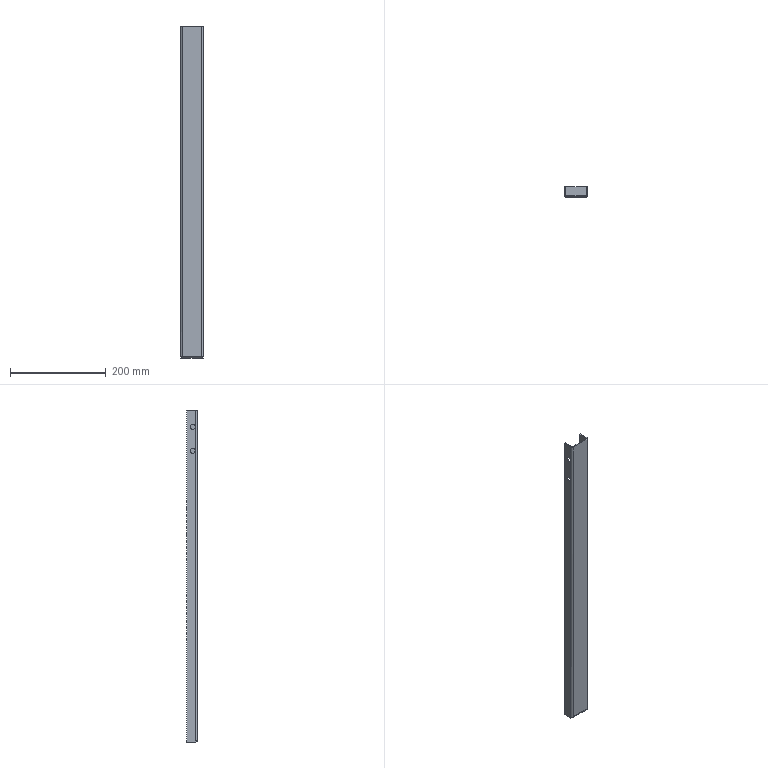Part | NX | features solid 2 | 1 solid | 34 faces | box 48 x 23 x 695 mm | volume 122908 mm3 | plane 24 | cylinder 10 | commonest cylinder face diameters 10 x4 4 x3 8 x3
STEP:
#1=CARTESIAN_POINT('',(1114.,-660.,1129.5));
#2=VERTEX_POINT('',#1);
#3=CARTESIAN_POINT('',(1114.,-670.,1129.5));
#4=VERTEX_POINT('',#3);
#5=CARTESIAN_POINT('',(1114.,-665.,1129.5));
#6=DIRECTION('',(1.,0.,0.));
#7=DIRECTION('',(0.,-1.,0.));
#8=AXIS2_PLACEMENT_3D('',#5,#6,#7);
#9=CIRCLE('',#8,5.);
#10=EDGE_CURVE('',#2,#4,#9,.T.);
#11=ORIENTED_EDGE('',*,*,#10,.F.);
#12=CARTESIAN_POINT('',(1114.,-665.,1129.5));
#13=DIRECTION('',(1.,0.,0.));
#14=DIRECTION('',(0.,-1.,0.));
#15=AXIS2_PLACEMENT_3D('',#12,#13,#14);
#16=CIRCLE('',#15,5.);
#17=EDGE_CURVE('',#4,#2,#16,.T.);
#18=ORIENTED_EDGE('',*,*,#17,.F.);
#19=EDGE_LOOP('',(#11,#18));
#20=FACE_BOUND('',#19,.T.);
#21=CARTESIAN_POINT('',(1114.,-660.,1079.5));
#22=VERTEX_POINT('',#21);
#23=CARTESIAN_POINT('',(1114.,-670.,1079.5));
#24=VERTEX_POINT('',#23);
#25=CARTESIAN_POINT('',(1114.,-665.,1079.5));
#26=DIRECTION('',(1.,0.,0.));
#27=DIRECTION('',(0.,-1.,0.));
#28=AXIS2_PLACEMENT_3D('',#25,#26,#27);
#29=CIRCLE('',#28,5.);
#30=EDGE_CURVE('',#22,#24,#29,.T.);
#31=ORIENTED_EDGE('',*,*,#30,.F.);
#32=CARTESIAN_POINT('',(1114.,-665.,1079.5));
#33=DIRECTION('',(1.,0.,0.));
#34=DIRECTION('',(0.,-1.,0.));
#35=AXIS2_PLACEMENT_3D('',#32,#33,#34);
#36=CIRCLE('',#35,5.);
#37=EDGE_CURVE('',#24,#22,#36,.T.);
#38=ORIENTED_EDGE('',*,*,#37,.F.);
#39=EDGE_LOOP('',(#31,#38));
#40=FACE_BOUND('',#39,.T.);
#41=CARTESIAN_POINT('',(1114.,-652.,470.));
#42=VERTEX_POINT('',#41);
#43=CARTESIAN_POINT('',(1114.,-671.,470.));
#44=VERTEX_POINT('',#43);
#45=CARTESIAN_POINT('',(1114.,-652.,470.));
#46=DIRECTION('',(0.,-1.,0.));
#47=VECTOR('',#46,1000.);
#48=LINE('',#45,#47);
#49=EDGE_CURVE('',#42,#44,#48,.T.);
#50=ORIENTED_EDGE('',*,*,#49,.F.);
#51=CARTESIAN_POINT('',(1114.,-652.,1165.));
#52=VERTEX_POINT('',#51);
#53=CARTESIAN_POINT('',(1114.,-652.,-140.));
#54=DIRECTION('',(0.,0.,1.));
#55=VECTOR('',#54,1000.);
#56=LINE('',#53,#55);
#57=EDGE_CURVE('',#42,#52,#56,.T.);
#58=ORIENTED_EDGE('',*,*,#57,.T.);
#59=CARTESIAN_POINT('',(1114.,-671.,1165.));
#60=VERTEX_POINT('',#59);
#61=CARTESIAN_POINT('',(1114.,-652.,1165.));
#62=DIRECTION('',(0.,1.,0.));
#63=VECTOR('',#62,1000.);
#64=LINE('',#61,#63);
#65=EDGE_CURVE('',#60,#52,#64,.T.);
#66=ORIENTED_EDGE('',*,*,#65,.F.);
#67=CARTESIAN_POINT('',(1114.,-671.,472.1));
#68=VERTEX_POINT('',#67);
#69=CARTESIAN_POINT('',(1114.,-671.,-140.));
#70=DIRECTION('',(0.,0.,1.));
#71=VECTOR('',#70,1000.);
#72=LINE('',#69,#71);
#73=EDGE_CURVE('',#68,#60,#72,.T.);
#74=ORIENTED_EDGE('',*,*,#73,.F.);
#75=CARTESIAN_POINT('',(1114.,-671.,-140.));
#76=DIRECTION('',(0.,0.,1.));
#77=VECTOR('',#76,1000.);
#78=LINE('',#75,#77);
#79=EDGE_CURVE('',#44,#68,#78,.T.);
#80=ORIENTED_EDGE('',*,*,#79,.F.);
#81=EDGE_LOOP('',(#50,#58,#66,#74,#80));
#82=FACE_BOUND('',#81,.T.);
#83=CARTESIAN_POINT('',(1114.,-652.,-140.));
#84=DIRECTION('',(1.,0.,0.));
#85=DIRECTION('',(0.,0.,1.));
#86=AXIS2_PLACEMENT_3D('',#83,#84,#85);
#87=PLANE('',#86);
#88=ADVANCED_FACE('',(#20,#40,#82),#87,.T.);
#89=CARTESIAN_POINT('',(1112.,-660.,1129.5));
#90=VERTEX_POINT('',#89);
#91=CARTESIAN_POINT('',(1112.,-670.,1129.5));
#92=VERTEX_POINT('',#91);
#93=CARTESIAN_POINT('',(1112.,-665.,1129.5));
#94=DIRECTION('',(1.,0.,0.));
#95=DIRECTION('',(0.,-1.,0.));
#96=AXIS2_PLACEMENT_3D('',#93,#94,#95);
#97=CIRCLE('',#96,5.);
#98=EDGE_CURVE('',#90,#92,#97,.T.);
#99=ORIENTED_EDGE('',*,*,#98,.T.);
#100=CARTESIAN_POINT('',(1112.,-665.,1129.5));
#101=DIRECTION('',(1.,0.,0.));
#102=DIRECTION('',(0.,-1.,0.));
#103=AXIS2_PLACEMENT_3D('',#100,#101,#102);
#104=CIRCLE('',#103,5.);
#105=EDGE_CURVE('',#92,#90,#104,.T.);
#106=ORIENTED_EDGE('',*,*,#105,.T.);
#107=EDGE_LOOP('',(#99,#106));
#108=FACE_BOUND('',#107,.T.);
#109=CARTESIAN_POINT('',(1112.,-660.,1079.5));
#110=VERTEX_POINT('',#109);
#111=CARTESIAN_POINT('',(1112.,-670.,1079.5));
#112=VERTEX_POINT('',#111);
#113=CARTESIAN_POINT('',(1112.,-665.,1079.5));
#114=DIRECTION('',(1.,0.,0.));
#115=DIRECTION('',(0.,-1.,0.));
#116=AXIS2_PLACEMENT_3D('',#113,#114,#115);
#117=CIRCLE('',#116,5.);
#118=EDGE_CURVE('',#110,#112,#117,.T.);
#119=ORIENTED_EDGE('',*,*,#118,.T.);
#120=CARTESIAN_POINT('',(1112.,-665.,1079.5));
#121=DIRECTION('',(1.,0.,0.));
#122=DIRECTION('',(0.,-1.,0.));
#123=AXIS2_PLACEMENT_3D('',#120,#121,#122);
#124=CIRCLE('',#123,5.);
#125=EDGE_CURVE('',#112,#110,#124,.T.);
#126=ORIENTED_EDGE('',*,*,#125,.T.);
#127=EDGE_LOOP('',(#119,#126));
#128=FACE_BOUND('',#127,.T.);
#129=CARTESIAN_POINT('',(1112.,-652.,470.));
#130=VERTEX_POINT('',#129);
#131=CARTESIAN_POINT('',(1112.,-652.,1165.));
#132=VERTEX_POINT('',#131);
#133=CARTESIAN_POINT('',(1112.,-652.,-140.));
#134=DIRECTION('',(0.,0.,1.));
#135=VECTOR('',#134,1000.);
#136=LINE('',#133,#135);
#137=EDGE_CURVE('',#130,#132,#136,.T.);
#138=ORIENTED_EDGE('',*,*,#137,.F.);
#139=CARTESIAN_POINT('',(1112.,-671.,470.));
#140=VERTEX_POINT('',#139);
#141=CARTESIAN_POINT('',(1112.,-652.,470.));
#142=DIRECTION('',(0.,-1.,0.));
#143=VECTOR('',#142,1000.);
#144=LINE('',#141,#143);
#145=EDGE_CURVE('',#130,#140,#144,.T.);
#146=ORIENTED_EDGE('',*,*,#145,.T.);
#147=CARTESIAN_POINT('',(1112.,-671.,472.1));
#148=VERTEX_POINT('',#147);
#149=CARTESIAN_POINT('',(1112.,-671.,-140.));
#150=DIRECTION('',(0.,0.,1.));
#151=VECTOR('',#150,1000.);
#152=LINE('',#149,#151);
#153=EDGE_CURVE('',#140,#148,#152,.T.);
#154=ORIENTED_EDGE('',*,*,#153,.T.);
#155=CARTESIAN_POINT('',(1112.,-671.,1165.));
#156=VERTEX_POINT('',#155);
#157=CARTESIAN_POINT('',(1112.,-671.,-140.));
#158=DIRECTION('',(0.,0.,1.));
#159=VECTOR('',#158,1000.);
#160=LINE('',#157,#159);
#161=EDGE_CURVE('',#148,#156,#160,.T.);
#162=ORIENTED_EDGE('',*,*,#161,.T.);
#163=CARTESIAN_POINT('',(1112.,-652.,1165.));
#164=DIRECTION('',(0.,1.,0.));
#165=VECTOR('',#164,1000.);
#166=LINE('',#163,#165);
#167=EDGE_CURVE('',#156,#132,#166,.T.);
#168=ORIENTED_EDGE('',*,*,#167,.T.);
#169=EDGE_LOOP('',(#138,#146,#154,#162,#168));
#170=FACE_BOUND('',#169,.T.);
#171=CARTESIAN_POINT('',(1112.,-652.,-140.));
#172=DIRECTION('',(1.,0.,0.));
#173=DIRECTION('',(0.,0.,1.));
#174=AXIS2_PLACEMENT_3D('',#171,#172,#173);
#175=PLANE('',#174);
#176=ADVANCED_FACE('',(#108,#128,#170),#175,.F.);
#177=ORIENTED_EDGE('',*,*,#49,.T.);
#178=CARTESIAN_POINT('',(1112.,-671.,470.));
#179=DIRECTION('',(1.,0.,0.));
#180=VECTOR('',#179,1000.);
#181=LINE('',#178,#180);
#182=EDGE_CURVE('',#140,#44,#181,.T.);
#183=ORIENTED_EDGE('',*,*,#182,.F.);
#184=ORIENTED_EDGE('',*,*,#145,.F.);
#185=CARTESIAN_POINT('',(1114.,-652.,470.));
#186=DIRECTION('',(1.,0.,0.));
#187=VECTOR('',#186,1000.);
#188=LINE('',#185,#187);
#189=EDGE_CURVE('',#130,#42,#188,.T.);
#190=ORIENTED_EDGE('',*,*,#189,.T.);
#191=EDGE_LOOP('',(#177,#183,#184,#190));
#192=FACE_BOUND('',#191,.T.);
#193=CARTESIAN_POINT('',(1158.,-673.,470.));
#194=DIRECTION('',(0.,0.,1.));
#195=DIRECTION('',(1.,0.,0.));
#196=AXIS2_PLACEMENT_3D('',#193,#194,#195);
#197=PLANE('',#196);
#198=ADVANCED_FACE('',(#192),#197,.F.);
#199=CARTESIAN_POINT('',(1110.,-670.,1079.5));
#200=DIRECTION('',(1.,0.,0.));
#201=VECTOR('',#200,1000.);
#202=LINE('',#199,#201);
#203=EDGE_CURVE('',#112,#24,#202,.T.);
#204=ORIENTED_EDGE('',*,*,#203,.F.);
#205=ORIENTED_EDGE('',*,*,#118,.F.);
#206=CARTESIAN_POINT('',(1110.,-660.,1079.5));
#207=DIRECTION('',(1.,0.,0.));
#208=VECTOR('',#207,1000.);
#209=LINE('',#206,#208);
#210=EDGE_CURVE('',#22,#110,#209,.F.);
#211=ORIENTED_EDGE('',*,*,#210,.F.);
#212=ORIENTED_EDGE('',*,*,#30,.T.);
#213=EDGE_LOOP('',(#204,#205,#211,#212));
#214=FACE_BOUND('',#213,.T.);
#215=CARTESIAN_POINT('',(1110.,-665.,1079.5));
#216=DIRECTION('',(1.,0.,0.));
#217=DIRECTION('',(0.,1.,0.));
#218=AXIS2_PLACEMENT_3D('',#215,#216,#217);
#219=CYLINDRICAL_SURFACE('',#218,5.);
#220=ADVANCED_FACE('',(#214),#219,.F.);
#221=CARTESIAN_POINT('',(1110.,-670.,1129.5));
#222=DIRECTION('',(1.,0.,0.));
#223=VECTOR('',#222,1000.);
#224=LINE('',#221,#223);
#225=EDGE_CURVE('',#4,#92,#224,.F.);
#226=ORIENTED_EDGE('',*,*,#225,.T.);
#227=ORIENTED_EDGE('',*,*,#98,.F.);
#228=CARTESIAN_POINT('',(1110.,-660.,1129.5));
#229=DIRECTION('',(1.,0.,0.));
#230=VECTOR('',#229,1000.);
#231=LINE('',#228,#230);
#232=EDGE_CURVE('',#90,#2,#231,.T.);
#233=ORIENTED_EDGE('',*,*,#232,.T.);
#234=ORIENTED_EDGE('',*,*,#10,.T.);
#235=EDGE_LOOP('',(#226,#227,#233,#234));
#236=FACE_BOUND('',#235,.T.);
#237=CARTESIAN_POINT('',(1110.,-665.,1129.5));
#238=DIRECTION('',(1.,0.,0.));
#239=DIRECTION('',(0.,1.,0.));
#240=AXIS2_PLACEMENT_3D('',#237,#238,#239);
#241=CYLINDRICAL_SURFACE('',#240,5.);
#242=ADVANCED_FACE('',(#236),#241,.F.);
#243=ORIENTED_EDGE('',*,*,#189,.F.);
#244=ORIENTED_EDGE('',*,*,#137,.T.);
#245=CARTESIAN_POINT('',(1114.,-652.,1165.));
#246=DIRECTION('',(1.,0.,0.));
#247=VECTOR('',#246,1000.);
#248=LINE('',#245,#247);
#249=EDGE_CURVE('',#132,#52,#248,.T.);
#250=ORIENTED_EDGE('',*,*,#249,.T.);
#251=ORIENTED_EDGE('',*,*,#57,.F.);
#252=EDGE_LOOP('',(#243,#244,#250,#251));
#253=FACE_BOUND('',#252,.T.);
#254=CARTESIAN_POINT('',(1114.,-652.,-140.));
#255=DIRECTION('',(0.,1.,0.));
#256=DIRECTION('',(0.,0.,-1.));
#257=AXIS2_PLACEMENT_3D('',#254,#255,#256);
#258=PLANE('',#257);
#259=ADVANCED_FACE('',(#253),#258,.T.);
#260=ORIENTED_EDGE('',*,*,#79,.T.);
#261=CARTESIAN_POINT('',(1136.,-671.,472.1));
#262=DIRECTION('',(-1.,0.,0.));
#263=VECTOR('',#262,1000.);
#264=LINE('',#261,#263);
#265=EDGE_CURVE('',#68,#148,#264,.T.);
#266=ORIENTED_EDGE('',*,*,#265,.T.);
#267=ORIENTED_EDGE('',*,*,#153,.F.);
#268=ORIENTED_EDGE('',*,*,#182,.T.);
#269=EDGE_LOOP('',(#260,#266,#267,#268));
#270=FACE_BOUND('',#269,.T.);
#271=CARTESIAN_POINT('',(1112.,-671.,-140.));
#272=DIRECTION('',(0.,1.,0.));
#273=DIRECTION('',(0.,0.,-1.));
#274=AXIS2_PLACEMENT_3D('',#271,#272,#273);
#275=PLANE('',#274);
#276=ADVANCED_FACE('',(#270),#275,.F.);
#277=CARTESIAN_POINT('',(1116.,-675.,1165.));
#278=VERTEX_POINT('',#277);
#279=CARTESIAN_POINT('',(1116.,-671.,1165.));
#280=DIRECTION('',(0.,0.,-1.));
#281=DIRECTION('',(0.,-1.,0.));
#282=AXIS2_PLACEMENT_3D('',#279,#280,#281);
#283=CIRCLE('',#282,4.);
#284=EDGE_CURVE('',#278,#156,#283,.T.);
#285=ORIENTED_EDGE('',*,*,#284,.F.);
#286=CARTESIAN_POINT('',(1156.,-675.,1165.));
#287=VERTEX_POINT('',#286);
#288=CARTESIAN_POINT('',(1114.,-675.,1165.));
#289=DIRECTION('',(-1.,0.,0.));
#290=VECTOR('',#289,1000.);
#291=LINE('',#288,#290);
#292=EDGE_CURVE('',#287,#278,#291,.T.);
#293=ORIENTED_EDGE('',*,*,#292,.F.);
#294=CARTESIAN_POINT('',(1160.,-671.,1165.));
#295=VERTEX_POINT('',#294);
#296=CARTESIAN_POINT('',(1156.,-671.,1165.));
#297=DIRECTION('',(0.,0.,-1.));
#298=DIRECTION('',(0.,-1.,0.));
#299=AXIS2_PLACEMENT_3D('',#296,#297,#298);
#300=CIRCLE('',#299,4.);
#301=EDGE_CURVE('',#295,#287,#300,.T.);
#302=ORIENTED_EDGE('',*,*,#301,.F.);
#303=CARTESIAN_POINT('',(1160.,-652.,1165.));
#304=VERTEX_POINT('',#303);
#305=CARTESIAN_POINT('',(1160.,-673.,1165.));
#306=DIRECTION('',(0.,-1.,0.));
#307=VECTOR('',#306,1000.);
#308=LINE('',#305,#307);
#309=EDGE_CURVE('',#304,#295,#308,.T.);
#310=ORIENTED_EDGE('',*,*,#309,.F.);
#311=CARTESIAN_POINT('',(1158.,-652.,1165.));
#312=VERTEX_POINT('',#311);
#313=CARTESIAN_POINT('',(1158.,-652.,1165.));
#314=DIRECTION('',(-1.,0.,0.));
#315=VECTOR('',#314,1000.);
#316=LINE('',#313,#315);
#317=EDGE_CURVE('',#304,#312,#316,.T.);
#318=ORIENTED_EDGE('',*,*,#317,.T.);
#319=CARTESIAN_POINT('',(1158.,-671.,1165.));
#320=VERTEX_POINT('',#319);
#321=CARTESIAN_POINT('',(1158.,-673.,1165.));
#322=DIRECTION('',(0.,-1.,0.));
#323=VECTOR('',#322,1000.);
#324=LINE('',#321,#323);
#325=EDGE_CURVE('',#312,#320,#324,.T.);
#326=ORIENTED_EDGE('',*,*,#325,.T.);
#327=CARTESIAN_POINT('',(1156.,-673.,1165.));
#328=VERTEX_POINT('',#327);
#329=CARTESIAN_POINT('',(1156.,-671.,1165.));
#330=DIRECTION('',(0.,0.,-1.));
#331=DIRECTION('',(0.,-1.,0.));
#332=AXIS2_PLACEMENT_3D('',#329,#330,#331);
#333=CIRCLE('',#332,2.);
#334=EDGE_CURVE('',#320,#328,#333,.T.);
#335=ORIENTED_EDGE('',*,*,#334,.T.);
#336=CARTESIAN_POINT('',(1116.,-673.,1165.));
#337=VERTEX_POINT('',#336);
#338=CARTESIAN_POINT('',(1114.,-673.,1165.));
#339=DIRECTION('',(-1.,0.,0.));
#340=VECTOR('',#339,1000.);
#341=LINE('',#338,#340);
#342=EDGE_CURVE('',#328,#337,#341,.T.);
#343=ORIENTED_EDGE('',*,*,#342,.T.);
#344=CARTESIAN_POINT('',(1116.,-671.,1165.));
#345=DIRECTION('',(0.,0.,-1.));
#346=DIRECTION('',(0.,-1.,0.));
#347=AXIS2_PLACEMENT_3D('',#344,#345,#346);
#348=CIRCLE('',#347,2.);
#349=EDGE_CURVE('',#337,#60,#348,.T.);
#350=ORIENTED_EDGE('',*,*,#349,.T.);
#351=ORIENTED_EDGE('',*,*,#65,.T.);
#352=ORIENTED_EDGE('',*,*,#249,.F.);
#353=ORIENTED_EDGE('',*,*,#167,.F.);
#354=EDGE_LOOP('',(#285,#293,#302,#310,#318,#326,#335,#343,#350,#351,#352,#353));
#355=FACE_BOUND('',#354,.T.);
#356=CARTESIAN_POINT('',(1158.,-673.,1165.));
#357=DIRECTION('',(0.,0.,-1.));
#358=DIRECTION('',(0.,-1.,0.));
#359=AXIS2_PLACEMENT_3D('',#356,#357,#358);
#360=PLANE('',#359);
#361=ADVANCED_FACE('',(#355),#360,.F.);
#362=CARTESIAN_POINT('',(1116.,-673.,474.));
#363=VERTEX_POINT('',#362);
#364=CARTESIAN_POINT('',(1116.,-673.,-140.));
#365=DIRECTION('',(0.,0.,1.));
#366=VECTOR('',#365,1000.);
#367=LINE('',#364,#366);
#368=EDGE_CURVE('',#363,#337,#367,.T.);
#369=ORIENTED_EDGE('',*,*,#368,.F.);
#370=CARTESIAN_POINT('',(1116.,-673.,474.));
#371=CARTESIAN_POINT('',(1114.828,-673.,472.887));
#372=CARTESIAN_POINT('',(1114.,-672.172,472.1));
#373=CARTESIAN_POINT('',(1114.,-671.,472.1));
#374=(BOUNDED_CURVE()B_SPLINE_CURVE(3,(#370,#371,#372,#373),.UNSPECIFIED.,.F.,.F.)B_SPLINE_CURVE_WITH_KNOTS((4,4),(1.571,3.142),.PIECEWISE_BEZIER_KNOTS.)CURVE()GEOMETRIC_REPRESENTATION_ITEM()RATIONAL_B_SPLINE_CURVE((1.,0.8047,0.8047,1.))REPRESENTATION_ITEM(''));
#375=EDGE_CURVE('',#363,#68,#374,.T.);
#376=ORIENTED_EDGE('',*,*,#375,.T.);
#377=ORIENTED_EDGE('',*,*,#73,.T.);
#378=ORIENTED_EDGE('',*,*,#349,.F.);
#379=EDGE_LOOP('',(#369,#376,#377,#378));
#380=FACE_BOUND('',#379,.T.);
#381=CARTESIAN_POINT('',(1116.,-671.,-140.));
#382=DIRECTION('',(0.,0.,1.));
#383=DIRECTION('',(0.,-1.,0.));
#384=AXIS2_PLACEMENT_3D('',#381,#382,#383);
#385=CYLINDRICAL_SURFACE('',#384,2.);
#386=ADVANCED_FACE('',(#380),#385,.F.);
#387=CARTESIAN_POINT('',(1116.,-675.,474.));
#388=VERTEX_POINT('',#387);
#389=CARTESIAN_POINT('',(1114.,-674.464,472.1));
#390=VERTEX_POINT('',#389);
#391=CARTESIAN_POINT('',(1116.,-675.,474.));
#392=CARTESIAN_POINT('',(1115.294,-675.,473.329));
#393=CARTESIAN_POINT('',(1114.612,-674.817,472.681));
#394=CARTESIAN_POINT('',(1114.,-674.464,472.1));
#395=(BOUNDED_CURVE()B_SPLINE_CURVE(3,(#391,#392,#393,#394),.UNSPECIFIED.,.F.,.F.)B_SPLINE_CURVE_WITH_KNOTS((4,4),(1.571,2.094),.PIECEWISE_BEZIER_KNOTS.)CURVE()GEOMETRIC_REPRESENTATION_ITEM()RATIONAL_B_SPLINE_CURVE((1.,0.9773,0.9773,1.))REPRESENTATION_ITEM(''));
#396=EDGE_CURVE('',#388,#390,#395,.T.);
#397=ORIENTED_EDGE('',*,*,#396,.F.);
#398=CARTESIAN_POINT('',(1116.,-675.,-140.));
#399=DIRECTION('',(0.,0.,1.));
#400=VECTOR('',#399,1000.);
#401=LINE('',#398,#400);
#402=EDGE_CURVE('',#388,#278,#401,.T.);
#403=ORIENTED_EDGE('',*,*,#402,.T.);
#404=ORIENTED_EDGE('',*,*,#284,.T.);
#405=ORIENTED_EDGE('',*,*,#161,.F.);
#406=CARTESIAN_POINT('',(1116.,-671.,472.1));
#407=DIRECTION('',(0.,0.,-1.));
#408=DIRECTION('',(0.,1.,0.));
#409=AXIS2_PLACEMENT_3D('',#406,#407,#408);
#410=CIRCLE('',#409,4.);
#411=EDGE_CURVE('',#390,#148,#410,.T.);
#412=ORIENTED_EDGE('',*,*,#411,.F.);
#413=EDGE_LOOP('',(#397,#403,#404,#405,#412));
#414=FACE_BOUND('',#413,.T.);
#415=CARTESIAN_POINT('',(1116.,-671.,-140.));
#416=DIRECTION('',(0.,0.,1.));
#417=DIRECTION('',(0.,-1.,0.));
#418=AXIS2_PLACEMENT_3D('',#415,#416,#417);
#419=CYLINDRICAL_SURFACE('',#418,4.);
#420=ADVANCED_FACE('',(#414),#419,.T.);
#421=CARTESIAN_POINT('',(1114.,325.,472.1));
#422=DIRECTION('',(0.,1.,0.));
#423=VECTOR('',#422,1000.);
#424=LINE('',#421,#423);
#425=EDGE_CURVE('',#390,#68,#424,.T.);
#426=ORIENTED_EDGE('',*,*,#425,.F.);
#427=ORIENTED_EDGE('',*,*,#411,.T.);
#428=ORIENTED_EDGE('',*,*,#265,.F.);
#429=EDGE_LOOP('',(#426,#427,#428));
#430=FACE_BOUND('',#429,.T.);
#431=CARTESIAN_POINT('',(1114.,-1675.,472.1));
#432=DIRECTION('',(0.,0.,-1.));
#433=DIRECTION('',(0.,-1.,0.));
#434=AXIS2_PLACEMENT_3D('',#431,#432,#433);
#435=PLANE('',#434);
#436=ADVANCED_FACE('',(#430),#435,.T.);
#437=CARTESIAN_POINT('',(1116.,-673.,474.));
#438=DIRECTION('',(0.,-1.,0.));
#439=VECTOR('',#438,1000.);
#440=LINE('',#437,#439);
#441=EDGE_CURVE('',#363,#388,#440,.T.);
#442=ORIENTED_EDGE('',*,*,#441,.T.);
#443=ORIENTED_EDGE('',*,*,#396,.T.);
#444=ORIENTED_EDGE('',*,*,#425,.T.);
#445=ORIENTED_EDGE('',*,*,#375,.F.);
#446=EDGE_LOOP('',(#442,#443,#444,#445));
#447=FACE_BOUND('',#446,.T.);
#448=CARTESIAN_POINT('',(1840.999,-1675.,1162.749));
#449=DIRECTION('',(0.6887,0.,-0.725));
#450=DIRECTION('',(0.,-1.,0.));
#451=AXIS2_PLACEMENT_3D('',#448,#449,#450);
#452=PLANE('',#451);
#453=ADVANCED_FACE('',(#447),#452,.T.);
#454=CARTESIAN_POINT('',(1157.9,-671.,472.));
#455=VERTEX_POINT('',#454);
#456=CARTESIAN_POINT('',(1114.1,-671.,472.));
#457=VERTEX_POINT('',#456);
#458=CARTESIAN_POINT('',(1156.,-671.,472.));
#459=DIRECTION('',(-1.,0.,0.));
#460=VECTOR('',#459,1000.);
#461=LINE('',#458,#460);
#462=EDGE_CURVE('',#455,#457,#461,.T.);
#463=ORIENTED_EDGE('',*,*,#462,.F.);
#464=CARTESIAN_POINT('',(1157.9,-652.,472.));
#465=VERTEX_POINT('',#464);
#466=CARTESIAN_POINT('',(1157.9,-673.278,472.));
#467=DIRECTION('',(0.,-1.,0.));
#468=VECTOR('',#467,1000.);
#469=LINE('',#466,#468);
#470=EDGE_CURVE('',#465,#455,#469,.T.);
#471=ORIENTED_EDGE('',*,*,#470,.F.);
#472=CARTESIAN_POINT('',(1114.1,-652.,472.));
#473=VERTEX_POINT('',#472);
#474=CARTESIAN_POINT('',(1116.,-652.,472.));
#475=DIRECTION('',(1.,0.,0.));
#476=VECTOR('',#475,1000.);
#477=LINE('',#474,#476);
#478=EDGE_CURVE('',#473,#465,#477,.T.);
#479=ORIENTED_EDGE('',*,*,#478,.F.);
#480=CARTESIAN_POINT('',(1114.1,-673.278,472.));
#481=DIRECTION('',(0.,1.,0.));
#482=VECTOR('',#481,1000.);
#483=LINE('',#480,#482);
#484=EDGE_CURVE('',#457,#473,#483,.T.);
#485=ORIENTED_EDGE('',*,*,#484,.F.);
#486=EDGE_LOOP('',(#463,#471,#479,#485));
#487=FACE_BOUND('',#486,.T.);
#488=CARTESIAN_POINT('',(1136.,-662.5,472.));
#489=DIRECTION('',(0.,0.,-1.));
#490=DIRECTION('',(0.,-1.,0.));
#491=AXIS2_PLACEMENT_3D('',#488,#489,#490);
#492=PLANE('',#491);
#493=ADVANCED_FACE('',(#487),#492,.F.);
#494=CARTESIAN_POINT('',(1157.9,-652.,470.));
#495=VERTEX_POINT('',#494);
#496=CARTESIAN_POINT('',(1157.9,-671.,470.));
#497=VERTEX_POINT('',#496);
#498=CARTESIAN_POINT('',(1157.9,-673.278,470.));
#499=DIRECTION('',(0.,-1.,0.));
#500=VECTOR('',#499,1000.);
#501=LINE('',#498,#500);
#502=EDGE_CURVE('',#495,#497,#501,.T.);
#503=ORIENTED_EDGE('',*,*,#502,.T.);
#504=CARTESIAN_POINT('',(1114.1,-671.,470.));
#505=VERTEX_POINT('',#504);
#506=CARTESIAN_POINT('',(1156.,-671.,470.));
#507=DIRECTION('',(-1.,0.,0.));
#508=VECTOR('',#507,1000.);
#509=LINE('',#506,#508);
#510=EDGE_CURVE('',#497,#505,#509,.T.);
#511=ORIENTED_EDGE('',*,*,#510,.T.);
#512=CARTESIAN_POINT('',(1114.1,-652.,470.));
#513=VERTEX_POINT('',#512);
#514=CARTESIAN_POINT('',(1114.1,-673.278,470.));
#515=DIRECTION('',(0.,1.,0.));
#516=VECTOR('',#515,1000.);
#517=LINE('',#514,#516);
#518=EDGE_CURVE('',#505,#513,#517,.T.);
#519=ORIENTED_EDGE('',*,*,#518,.T.);
#520=CARTESIAN_POINT('',(1116.,-652.,470.));
#521=DIRECTION('',(1.,0.,0.));
#522=VECTOR('',#521,1000.);
#523=LINE('',#520,#522);
#524=EDGE_CURVE('',#513,#495,#523,.T.);
#525=ORIENTED_EDGE('',*,*,#524,.T.);
#526=EDGE_LOOP('',(#503,#511,#519,#525));
#527=FACE_BOUND('',#526,.T.);
#528=CARTESIAN_POINT('',(1136.,-662.5,470.));
#529=DIRECTION('',(0.,0.,-1.));
#530=DIRECTION('',(0.,-1.,0.));
#531=AXIS2_PLACEMENT_3D('',#528,#529,#530);
#532=PLANE('',#531);
#533=ADVANCED_FACE('',(#527),#532,.T.);
#534=ORIENTED_EDGE('',*,*,#478,.T.);
#535=CARTESIAN_POINT('',(1157.9,-652.,470.));
#536=DIRECTION('',(0.,0.,1.));
#537=VECTOR('',#536,1000.);
#538=LINE('',#535,#537);
#539=EDGE_CURVE('',#495,#465,#538,.T.);
#540=ORIENTED_EDGE('',*,*,#539,.F.);
#541=ORIENTED_EDGE('',*,*,#524,.F.);
#542=CARTESIAN_POINT('',(1114.1,-652.,470.));
#543=DIRECTION('',(0.,0.,1.));
#544=VECTOR('',#543,1000.);
#545=LINE('',#542,#544);
#546=EDGE_CURVE('',#513,#473,#545,.T.);
#547=ORIENTED_EDGE('',*,*,#546,.T.);
#548=EDGE_LOOP('',(#534,#540,#541,#547));
#549=FACE_BOUND('',#548,.T.);
#550=CARTESIAN_POINT('',(1116.,-652.,470.));
#551=DIRECTION('',(0.,-1.,0.));
#552=DIRECTION('',(-1.,0.,0.));
#553=AXIS2_PLACEMENT_3D('',#550,#551,#552);
#554=PLANE('',#553);
#555=ADVANCED_FACE('',(#549),#554,.F.);
#556=CARTESIAN_POINT('',(1114.1,-671.,472.));
#557=CARTESIAN_POINT('',(1114.1,-672.172,472.));
#558=CARTESIAN_POINT('',(1114.887,-673.,472.828));
#559=CARTESIAN_POINT('',(1116.,-673.,474.));
#560=(BOUNDED_CURVE()B_SPLINE_CURVE(3,(#556,#557,#558,#559),.UNSPECIFIED.,.F.,.F.)B_SPLINE_CURVE_WITH_KNOTS((4,4),(3.142,4.712),.PIECEWISE_BEZIER_KNOTS.)CURVE()GEOMETRIC_REPRESENTATION_ITEM()RATIONAL_B_SPLINE_CURVE((1.,0.8047,0.8047,1.))REPRESENTATION_ITEM(''));
#561=EDGE_CURVE('',#457,#363,#560,.T.);
#562=ORIENTED_EDGE('',*,*,#561,.F.);
#563=CARTESIAN_POINT('',(1114.1,-674.464,472.));
#564=VERTEX_POINT('',#563);
#565=CARTESIAN_POINT('',(1114.1,325.,472.));
#566=DIRECTION('',(0.,1.,0.));
#567=VECTOR('',#566,1000.);
#568=LINE('',#565,#567);
#569=EDGE_CURVE('',#564,#457,#568,.T.);
#570=ORIENTED_EDGE('',*,*,#569,.F.);
#571=CARTESIAN_POINT('',(1114.1,-674.464,472.));
#572=CARTESIAN_POINT('',(1114.681,-674.817,472.612));
#573=CARTESIAN_POINT('',(1115.329,-675.,473.294));
#574=CARTESIAN_POINT('',(1116.,-675.,474.));
#575=(BOUNDED_CURVE()B_SPLINE_CURVE(3,(#571,#572,#573,#574),.UNSPECIFIED.,.F.,.F.)B_SPLINE_CURVE_WITH_KNOTS((4,4),(4.189,4.712),.PIECEWISE_BEZIER_KNOTS.)CURVE()GEOMETRIC_REPRESENTATION_ITEM()RATIONAL_B_SPLINE_CURVE((1.,0.9773,0.9773,1.))REPRESENTATION_ITEM(''));
#576=EDGE_CURVE('',#564,#388,#575,.T.);
#577=ORIENTED_EDGE('',*,*,#576,.T.);
#578=ORIENTED_EDGE('',*,*,#441,.F.);
#579=EDGE_LOOP('',(#562,#570,#577,#578));
#580=FACE_BOUND('',#579,.T.);
#581=CARTESIAN_POINT('',(1804.749,-1675.,1198.999));
#582=DIRECTION('',(0.725,0.,-0.6887));
#583=DIRECTION('',(0.,-1.,0.));
#584=AXIS2_PLACEMENT_3D('',#581,#582,#583);
#585=PLANE('',#584);
#586=ADVANCED_FACE('',(#580),#585,.F.);
#587=ORIENTED_EDGE('',*,*,#569,.T.);
#588=ORIENTED_EDGE('',*,*,#484,.T.);
#589=ORIENTED_EDGE('',*,*,#546,.F.);
#590=ORIENTED_EDGE('',*,*,#518,.F.);
#591=CARTESIAN_POINT('',(1114.1,-671.,474.));
#592=DIRECTION('',(-1.,0.,0.));
#593=DIRECTION('',(0.,-1.,0.));
#594=AXIS2_PLACEMENT_3D('',#591,#592,#593);
#595=CIRCLE('',#594,4.);
#596=EDGE_CURVE('',#505,#564,#595,.T.);
#597=ORIENTED_EDGE('',*,*,#596,.T.);
#598=EDGE_LOOP('',(#587,#588,#589,#590,#597));
#599=FACE_BOUND('',#598,.T.);
#600=CARTESIAN_POINT('',(1114.1,-1675.,472.));
#601=DIRECTION('',(1.,0.,0.));
#602=DIRECTION('',(0.,0.,1.));
#603=AXIS2_PLACEMENT_3D('',#600,#601,#602);
#604=PLANE('',#603);
#605=ADVANCED_FACE('',(#599),#604,.F.);
#606=CARTESIAN_POINT('',(1157.9,-674.464,472.));
#607=VERTEX_POINT('',#606);
#608=CARTESIAN_POINT('',(1156.,-675.,474.));
#609=VERTEX_POINT('',#608);
#610=CARTESIAN_POINT('',(1157.9,-674.464,472.));
#611=CARTESIAN_POINT('',(1157.319,-674.817,472.612));
#612=CARTESIAN_POINT('',(1156.671,-675.,473.294));
#613=CARTESIAN_POINT('',(1156.,-675.,474.));
#614=(BOUNDED_CURVE()B_SPLINE_CURVE(3,(#610,#611,#612,#613),.UNSPECIFIED.,.F.,.F.)B_SPLINE_CURVE_WITH_KNOTS((4,4),(1.047,1.571),.PIECEWISE_BEZIER_KNOTS.)CURVE()GEOMETRIC_REPRESENTATION_ITEM()RATIONAL_B_SPLINE_CURVE((1.,0.9773,0.9773,1.))REPRESENTATION_ITEM(''));
#615=EDGE_CURVE('',#607,#609,#614,.T.);
#616=ORIENTED_EDGE('',*,*,#615,.F.);
#617=CARTESIAN_POINT('',(1157.9,325.,472.));
#618=DIRECTION('',(0.,1.,0.));
#619=VECTOR('',#618,1000.);
#620=LINE('',#617,#619);
#621=EDGE_CURVE('',#607,#455,#620,.T.);
#622=ORIENTED_EDGE('',*,*,#621,.T.);
#623=CARTESIAN_POINT('',(1156.,-673.,474.));
#624=VERTEX_POINT('',#623);
#625=CARTESIAN_POINT('',(1157.9,-671.,472.));
#626=CARTESIAN_POINT('',(1157.9,-672.172,472.));
#627=CARTESIAN_POINT('',(1157.113,-673.,472.828));
#628=CARTESIAN_POINT('',(1156.,-673.,474.));
#629=(BOUNDED_CURVE()B_SPLINE_CURVE(3,(#625,#626,#627,#628),.UNSPECIFIED.,.F.,.F.)B_SPLINE_CURVE_WITH_KNOTS((4,4),(0.,1.571),.PIECEWISE_BEZIER_KNOTS.)CURVE()GEOMETRIC_REPRESENTATION_ITEM()RATIONAL_B_SPLINE_CURVE((1.,0.8047,0.8047,1.))REPRESENTATION_ITEM(''));
#630=EDGE_CURVE('',#455,#624,#629,.T.);
#631=ORIENTED_EDGE('',*,*,#630,.T.);
#632=CARTESIAN_POINT('',(1156.,-673.,474.));
#633=DIRECTION('',(0.,-1.,0.));
#634=VECTOR('',#633,1000.);
#635=LINE('',#632,#634);
#636=EDGE_CURVE('',#624,#609,#635,.T.);
#637=ORIENTED_EDGE('',*,*,#636,.T.);
#638=EDGE_LOOP('',(#616,#622,#631,#637));
#639=FACE_BOUND('',#638,.T.);
#640=CARTESIAN_POINT('',(467.251,-1675.,1198.999));
#641=DIRECTION('',(0.725,0.,0.6887));
#642=DIRECTION('',(0.,-1.,0.));
#643=AXIS2_PLACEMENT_3D('',#640,#641,#642);
#644=PLANE('',#643);
#645=ADVANCED_FACE('',(#639),#644,.T.);
#646=ORIENTED_EDGE('',*,*,#576,.F.);
#647=ORIENTED_EDGE('',*,*,#596,.F.);
#648=ORIENTED_EDGE('',*,*,#510,.F.);
#649=CARTESIAN_POINT('',(1157.9,-671.,474.));
#650=DIRECTION('',(-1.,0.,0.));
#651=DIRECTION('',(0.,-1.,0.));
#652=AXIS2_PLACEMENT_3D('',#649,#650,#651);
#653=CIRCLE('',#652,4.);
#654=EDGE_CURVE('',#497,#607,#653,.T.);
#655=ORIENTED_EDGE('',*,*,#654,.T.);
#656=ORIENTED_EDGE('',*,*,#615,.T.);
#657=CARTESIAN_POINT('',(1116.,-675.,474.));
#658=DIRECTION('',(1.,0.,0.));
#659=VECTOR('',#658,1000.);
#660=LINE('',#657,#659);
#661=EDGE_CURVE('',#388,#609,#660,.T.);
#662=ORIENTED_EDGE('',*,*,#661,.F.);
#663=EDGE_LOOP('',(#646,#647,#648,#655,#656,#662));
#664=FACE_BOUND('',#663,.T.);
#665=CARTESIAN_POINT('',(1116.,-671.,474.));
#666=DIRECTION('',(1.,0.,0.));
#667=DIRECTION('',(0.,1.,0.));
#668=AXIS2_PLACEMENT_3D('',#665,#666,#667);
#669=CYLINDRICAL_SURFACE('',#668,4.);
#670=ADVANCED_FACE('',(#664),#669,.T.);
#671=ORIENTED_EDGE('',*,*,#654,.F.);
#672=ORIENTED_EDGE('',*,*,#502,.F.);
#673=ORIENTED_EDGE('',*,*,#539,.T.);
#674=ORIENTED_EDGE('',*,*,#470,.T.);
#675=ORIENTED_EDGE('',*,*,#621,.F.);
#676=EDGE_LOOP('',(#671,#672,#673,#674,#675));
#677=FACE_BOUND('',#676,.T.);
#678=CARTESIAN_POINT('',(1157.9,-1675.,472.));
#679=DIRECTION('',(1.,0.,0.));
#680=DIRECTION('',(0.,0.,1.));
#681=AXIS2_PLACEMENT_3D('',#678,#679,#680);
#682=PLANE('',#681);
#683=ADVANCED_FACE('',(#677),#682,.T.);
#684=ORIENTED_EDGE('',*,*,#462,.T.);
#685=ORIENTED_EDGE('',*,*,#561,.T.);
#686=CARTESIAN_POINT('',(1116.,-673.,474.));
#687=DIRECTION('',(1.,0.,0.));
#688=VECTOR('',#687,1000.);
#689=LINE('',#686,#688);
#690=EDGE_CURVE('',#363,#624,#689,.T.);
#691=ORIENTED_EDGE('',*,*,#690,.T.);
#692=ORIENTED_EDGE('',*,*,#630,.F.);
#693=EDGE_LOOP('',(#684,#685,#691,#692));
#694=FACE_BOUND('',#693,.T.);
#695=CARTESIAN_POINT('',(1116.,-671.,474.));
#696=DIRECTION('',(1.,0.,0.));
#697=DIRECTION('',(0.,1.,0.));
#698=AXIS2_PLACEMENT_3D('',#695,#696,#697);
#699=CYLINDRICAL_SURFACE('',#698,2.);
#700=ADVANCED_FACE('',(#694),#699,.F.);
#701=CARTESIAN_POINT('',(1160.,-671.,470.));
#702=VERTEX_POINT('',#701);
#703=CARTESIAN_POINT('',(1160.,-671.,472.1));
#704=VERTEX_POINT('',#703);
#705=CARTESIAN_POINT('',(1160.,-671.,-140.));
#706=DIRECTION('',(0.,0.,1.));
#707=VECTOR('',#706,1000.);
#708=LINE('',#705,#707);
#709=EDGE_CURVE('',#702,#704,#708,.T.);
#710=ORIENTED_EDGE('',*,*,#709,.F.);
#711=CARTESIAN_POINT('',(1160.,-652.,470.));
#712=VERTEX_POINT('',#711);
#713=CARTESIAN_POINT('',(1160.,-673.,470.));
#714=DIRECTION('',(0.,1.,0.));
#715=VECTOR('',#714,1000.);
#716=LINE('',#713,#715);
#717=EDGE_CURVE('',#702,#712,#716,.T.);
#718=ORIENTED_EDGE('',*,*,#717,.T.);
#719=CARTESIAN_POINT('',(1160.,-652.,-140.));
#720=DIRECTION('',(0.,0.,1.));
#721=VECTOR('',#720,1000.);
#722=LINE('',#719,#721);
#723=EDGE_CURVE('',#712,#304,#722,.T.);
#724=ORIENTED_EDGE('',*,*,#723,.T.);
#725=ORIENTED_EDGE('',*,*,#309,.T.);
#726=CARTESIAN_POINT('',(1160.,-671.,-140.));
#727=DIRECTION('',(0.,0.,1.));
#728=VECTOR('',#727,1000.);
#729=LINE('',#726,#728);
#730=EDGE_CURVE('',#704,#295,#729,.T.);
#731=ORIENTED_EDGE('',*,*,#730,.F.);
#732=EDGE_LOOP('',(#710,#718,#724,#725,#731));
#733=FACE_BOUND('',#732,.T.);
#734=CARTESIAN_POINT('',(1160.,-673.,-140.));
#735=DIRECTION('',(-1.,0.,0.));
#736=DIRECTION('',(0.,0.,1.));
#737=AXIS2_PLACEMENT_3D('',#734,#735,#736);
#738=PLANE('',#737);
#739=ADVANCED_FACE('',(#733),#738,.F.);
#740=CARTESIAN_POINT('',(1158.,-671.,470.));
#741=VERTEX_POINT('',#740);
#742=CARTESIAN_POINT('',(1158.,-652.,470.));
#743=VERTEX_POINT('',#742);
#744=CARTESIAN_POINT('',(1158.,-673.,470.));
#745=DIRECTION('',(0.,1.,0.));
#746=VECTOR('',#745,1000.);
#747=LINE('',#744,#746);
#748=EDGE_CURVE('',#741,#743,#747,.T.);
#749=ORIENTED_EDGE('',*,*,#748,.F.);
#750=CARTESIAN_POINT('',(1158.,-671.,472.1));
#751=VERTEX_POINT('',#750);
#752=CARTESIAN_POINT('',(1158.,-671.,-140.));
#753=DIRECTION('',(0.,0.,1.));
#754=VECTOR('',#753,1000.);
#755=LINE('',#752,#754);
#756=EDGE_CURVE('',#741,#751,#755,.T.);
#757=ORIENTED_EDGE('',*,*,#756,.T.);
#758=CARTESIAN_POINT('',(1158.,-671.,-140.));
#759=DIRECTION('',(0.,0.,1.));
#760=VECTOR('',#759,1000.);
#761=LINE('',#758,#760);
#762=EDGE_CURVE('',#751,#320,#761,.T.);
#763=ORIENTED_EDGE('',*,*,#762,.T.);
#764=ORIENTED_EDGE('',*,*,#325,.F.);
#765=CARTESIAN_POINT('',(1158.,-652.,-140.));
#766=DIRECTION('',(0.,0.,1.));
#767=VECTOR('',#766,1000.);
#768=LINE('',#765,#767);
#769=EDGE_CURVE('',#743,#312,#768,.T.);
#770=ORIENTED_EDGE('',*,*,#769,.F.);
#771=EDGE_LOOP('',(#749,#757,#763,#764,#770));
#772=FACE_BOUND('',#771,.T.);
#773=CARTESIAN_POINT('',(1158.,-673.,-140.));
#774=DIRECTION('',(-1.,0.,0.));
#775=DIRECTION('',(0.,0.,1.));
#776=AXIS2_PLACEMENT_3D('',#773,#774,#775);
#777=PLANE('',#776);
#778=ADVANCED_FACE('',(#772),#777,.T.);
#779=ORIENTED_EDGE('',*,*,#709,.T.);
#780=CARTESIAN_POINT('',(1136.,-671.,472.1));
#781=DIRECTION('',(-1.,0.,0.));
#782=VECTOR('',#781,1000.);
#783=LINE('',#780,#782);
#784=EDGE_CURVE('',#704,#751,#783,.T.);
#785=ORIENTED_EDGE('',*,*,#784,.T.);
#786=ORIENTED_EDGE('',*,*,#756,.F.);
#787=CARTESIAN_POINT('',(1160.,-671.,470.));
#788=DIRECTION('',(-1.,0.,0.));
#789=VECTOR('',#788,1000.);
#790=LINE('',#787,#789);
#791=EDGE_CURVE('',#702,#741,#790,.T.);
#792=ORIENTED_EDGE('',*,*,#791,.F.);
#793=EDGE_LOOP('',(#779,#785,#786,#792));
#794=FACE_BOUND('',#793,.T.);
#795=CARTESIAN_POINT('',(1160.,-671.,-140.));
#796=DIRECTION('',(0.,-1.,0.));
#797=DIRECTION('',(-1.,0.,0.));
#798=AXIS2_PLACEMENT_3D('',#795,#796,#797);
#799=PLANE('',#798);
#800=ADVANCED_FACE('',(#794),#799,.T.);
#801=ORIENTED_EDGE('',*,*,#791,.T.);
#802=ORIENTED_EDGE('',*,*,#748,.T.);
#803=CARTESIAN_POINT('',(1158.,-652.,470.));
#804=DIRECTION('',(-1.,0.,0.));
#805=VECTOR('',#804,1000.);
#806=LINE('',#803,#805);
#807=EDGE_CURVE('',#712,#743,#806,.T.);
#808=ORIENTED_EDGE('',*,*,#807,.F.);
#809=ORIENTED_EDGE('',*,*,#717,.F.);
#810=EDGE_LOOP('',(#801,#802,#808,#809));
#811=FACE_BOUND('',#810,.T.);
#812=CARTESIAN_POINT('',(1158.,-673.,470.));
#813=DIRECTION('',(0.,0.,1.));
#814=DIRECTION('',(1.,0.,0.));
#815=AXIS2_PLACEMENT_3D('',#812,#813,#814);
#816=PLANE('',#815);
#817=ADVANCED_FACE('',(#811),#816,.F.);
#818=ORIENTED_EDGE('',*,*,#723,.F.);
#819=ORIENTED_EDGE('',*,*,#807,.T.);
#820=ORIENTED_EDGE('',*,*,#769,.T.);
#821=ORIENTED_EDGE('',*,*,#317,.F.);
#822=EDGE_LOOP('',(#818,#819,#820,#821));
#823=FACE_BOUND('',#822,.T.);
#824=CARTESIAN_POINT('',(1158.,-652.,-140.));
#825=DIRECTION('',(0.,-1.,0.));
#826=DIRECTION('',(-1.,0.,0.));
#827=AXIS2_PLACEMENT_3D('',#824,#825,#826);
#828=PLANE('',#827);
#829=ADVANCED_FACE('',(#823),#828,.F.);
#830=ORIENTED_EDGE('',*,*,#636,.F.);
#831=CARTESIAN_POINT('',(1156.,-673.,474.));
#832=CARTESIAN_POINT('',(1157.172,-673.,472.887));
#833=CARTESIAN_POINT('',(1158.,-672.172,472.1));
#834=CARTESIAN_POINT('',(1158.,-671.,472.1));
#835=(BOUNDED_CURVE()B_SPLINE_CURVE(3,(#831,#832,#833,#834),.UNSPECIFIED.,.F.,.F.)B_SPLINE_CURVE_WITH_KNOTS((4,4),(1.571,3.142),.PIECEWISE_BEZIER_KNOTS.)CURVE()GEOMETRIC_REPRESENTATION_ITEM()RATIONAL_B_SPLINE_CURVE((1.,0.8047,0.8047,1.))REPRESENTATION_ITEM(''));
#836=EDGE_CURVE('',#624,#751,#835,.T.);
#837=ORIENTED_EDGE('',*,*,#836,.T.);
#838=CARTESIAN_POINT('',(1158.,-674.464,472.1));
#839=VERTEX_POINT('',#838);
#840=CARTESIAN_POINT('',(1158.,325.,472.1));
#841=DIRECTION('',(0.,1.,0.));
#842=VECTOR('',#841,1000.);
#843=LINE('',#840,#842);
#844=EDGE_CURVE('',#839,#751,#843,.T.);
#845=ORIENTED_EDGE('',*,*,#844,.F.);
#846=CARTESIAN_POINT('',(1156.,-675.,474.));
#847=CARTESIAN_POINT('',(1156.706,-675.,473.329));
#848=CARTESIAN_POINT('',(1157.388,-674.817,472.681));
#849=CARTESIAN_POINT('',(1158.,-674.464,472.1));
#850=(BOUNDED_CURVE()B_SPLINE_CURVE(3,(#846,#847,#848,#849),.UNSPECIFIED.,.F.,.F.)B_SPLINE_CURVE_WITH_KNOTS((4,4),(1.571,2.094),.PIECEWISE_BEZIER_KNOTS.)CURVE()GEOMETRIC_REPRESENTATION_ITEM()RATIONAL_B_SPLINE_CURVE((1.,0.9773,0.9773,1.))REPRESENTATION_ITEM(''));
#851=EDGE_CURVE('',#609,#839,#850,.T.);
#852=ORIENTED_EDGE('',*,*,#851,.F.);
#853=EDGE_LOOP('',(#830,#837,#845,#852));
#854=FACE_BOUND('',#853,.T.);
#855=CARTESIAN_POINT('',(431.001,-1675.,1162.749));
#856=DIRECTION('',(0.6887,0.,0.725));
#857=DIRECTION('',(0.,-1.,0.));
#858=AXIS2_PLACEMENT_3D('',#855,#856,#857);
#859=PLANE('',#858);
#860=ADVANCED_FACE('',(#854),#859,.F.);
#861=CARTESIAN_POINT('',(1156.,-671.,472.1));
#862=DIRECTION('',(0.,0.,1.));
#863=DIRECTION('',(0.,-1.,0.));
#864=AXIS2_PLACEMENT_3D('',#861,#862,#863);
#865=CIRCLE('',#864,4.);
#866=EDGE_CURVE('',#839,#704,#865,.T.);
#867=ORIENTED_EDGE('',*,*,#866,.F.);
#868=ORIENTED_EDGE('',*,*,#844,.T.);
#869=ORIENTED_EDGE('',*,*,#784,.F.);
#870=EDGE_LOOP('',(#867,#868,#869));
#871=FACE_BOUND('',#870,.T.);
#872=CARTESIAN_POINT('',(1158.,-1675.,472.1));
#873=DIRECTION('',(0.,0.,1.));
#874=DIRECTION('',(1.,0.,0.));
#875=AXIS2_PLACEMENT_3D('',#872,#873,#874);
#876=PLANE('',#875);
#877=ADVANCED_FACE('',(#871),#876,.F.);
#878=CARTESIAN_POINT('',(1156.,-675.,-140.));
#879=DIRECTION('',(0.,0.,1.));
#880=VECTOR('',#879,1000.);
#881=LINE('',#878,#880);
#882=EDGE_CURVE('',#609,#287,#881,.T.);
#883=ORIENTED_EDGE('',*,*,#882,.F.);
#884=ORIENTED_EDGE('',*,*,#851,.T.);
#885=ORIENTED_EDGE('',*,*,#866,.T.);
#886=ORIENTED_EDGE('',*,*,#730,.T.);
#887=ORIENTED_EDGE('',*,*,#301,.T.);
#888=EDGE_LOOP('',(#883,#884,#885,#886,#887));
#889=FACE_BOUND('',#888,.T.);
#890=CARTESIAN_POINT('',(1156.,-671.,-140.));
#891=DIRECTION('',(0.,0.,1.));
#892=DIRECTION('',(0.,-1.,0.));
#893=AXIS2_PLACEMENT_3D('',#890,#891,#892);
#894=CYLINDRICAL_SURFACE('',#893,4.);
#895=ADVANCED_FACE('',(#889),#894,.T.);
#896=ORIENTED_EDGE('',*,*,#836,.F.);
#897=CARTESIAN_POINT('',(1156.,-673.,-140.));
#898=DIRECTION('',(0.,0.,1.));
#899=VECTOR('',#898,1000.);
#900=LINE('',#897,#899);
#901=EDGE_CURVE('',#624,#328,#900,.T.);
#902=ORIENTED_EDGE('',*,*,#901,.T.);
#903=ORIENTED_EDGE('',*,*,#334,.F.);
#904=ORIENTED_EDGE('',*,*,#762,.F.);
#905=EDGE_LOOP('',(#896,#902,#903,#904));
#906=FACE_BOUND('',#905,.T.);
#907=CARTESIAN_POINT('',(1156.,-671.,-140.));
#908=DIRECTION('',(0.,0.,1.));
#909=DIRECTION('',(0.,-1.,0.));
#910=AXIS2_PLACEMENT_3D('',#907,#908,#909);
#911=CYLINDRICAL_SURFACE('',#910,2.);
#912=ADVANCED_FACE('',(#906),#911,.F.);
#913=ORIENTED_EDGE('',*,*,#690,.F.);
#914=ORIENTED_EDGE('',*,*,#368,.T.);
#915=ORIENTED_EDGE('',*,*,#342,.F.);
#916=ORIENTED_EDGE('',*,*,#901,.F.);
#917=EDGE_LOOP('',(#913,#914,#915,#916));
#918=FACE_BOUND('',#917,.T.);
#919=CARTESIAN_POINT('',(1114.,-673.,-140.));
#920=DIRECTION('',(0.,1.,0.));
#921=DIRECTION('',(0.,0.,-1.));
#922=AXIS2_PLACEMENT_3D('',#919,#920,#921);
#923=PLANE('',#922);
#924=ADVANCED_FACE('',(#918),#923,.T.);
#925=ORIENTED_EDGE('',*,*,#402,.F.);
#926=ORIENTED_EDGE('',*,*,#661,.T.);
#927=ORIENTED_EDGE('',*,*,#882,.T.);
#928=ORIENTED_EDGE('',*,*,#292,.T.);
#929=EDGE_LOOP('',(#925,#926,#927,#928));
#930=FACE_BOUND('',#929,.T.);
#931=CARTESIAN_POINT('',(1114.,-675.,-140.));
#932=DIRECTION('',(0.,1.,0.));
#933=DIRECTION('',(0.,0.,-1.));
#934=AXIS2_PLACEMENT_3D('',#931,#932,#933);
#935=PLANE('',#934);
#936=ADVANCED_FACE('',(#930),#935,.F.);
#937=ORIENTED_EDGE('',*,*,#105,.F.);
#938=ORIENTED_EDGE('',*,*,#225,.F.);
#939=ORIENTED_EDGE('',*,*,#17,.T.);
#940=ORIENTED_EDGE('',*,*,#232,.F.);
#941=EDGE_LOOP('',(#937,#938,#939,#940));
#942=FACE_BOUND('',#941,.T.);
#943=CARTESIAN_POINT('',(1110.,-665.,1129.5));
#944=DIRECTION('',(1.,0.,0.));
#945=DIRECTION('',(0.,1.,0.));
#946=AXIS2_PLACEMENT_3D('',#943,#944,#945);
#947=CYLINDRICAL_SURFACE('',#946,5.);
#948=ADVANCED_FACE('',(#942),#947,.F.);
#949=ORIENTED_EDGE('',*,*,#125,.F.);
#950=ORIENTED_EDGE('',*,*,#203,.T.);
#951=ORIENTED_EDGE('',*,*,#37,.T.);
#952=ORIENTED_EDGE('',*,*,#210,.T.);
#953=EDGE_LOOP('',(#949,#950,#951,#952));
#954=FACE_BOUND('',#953,.T.);
#955=CARTESIAN_POINT('',(1110.,-665.,1079.5));
#956=DIRECTION('',(1.,0.,0.));
#957=DIRECTION('',(0.,1.,0.));
#958=AXIS2_PLACEMENT_3D('',#955,#956,#957);
#959=CYLINDRICAL_SURFACE('',#958,5.);
#960=ADVANCED_FACE('',(#954),#959,.F.);
#961=CLOSED_SHELL('',(#88,#176,#198,#220,#242,#259,#276,#361,#386,#420,#436,#453,#493,#533,#555,#586,#605,#645,#670,#683,#700,#739,#778,#800,#817,#829,#860,#877,#895,#912,#924,#936,#948,#960));
#962=MANIFOLD_SOLID_BREP('',#961);
#963=(LENGTH_UNIT()NAMED_UNIT(*)SI_UNIT(.MILLI.,.METRE.));
#964=UNCERTAINTY_MEASURE_WITH_UNIT(LENGTH_MEASURE(0.00001),#963,'','');
#965=(NAMED_UNIT(*)PLANE_ANGLE_UNIT()SI_UNIT($,.RADIAN.));
#966=(NAMED_UNIT(*)SI_UNIT($,.STERADIAN.)SOLID_ANGLE_UNIT());
#967=(GEOMETRIC_REPRESENTATION_CONTEXT(3)GLOBAL_UNCERTAINTY_ASSIGNED_CONTEXT((#964))GLOBAL_UNIT_ASSIGNED_CONTEXT((#963,#965,#966))REPRESENTATION_CONTEXT('',''));
#968=ADVANCED_BREP_SHAPE_REPRESENTATION('',(#962),#967);